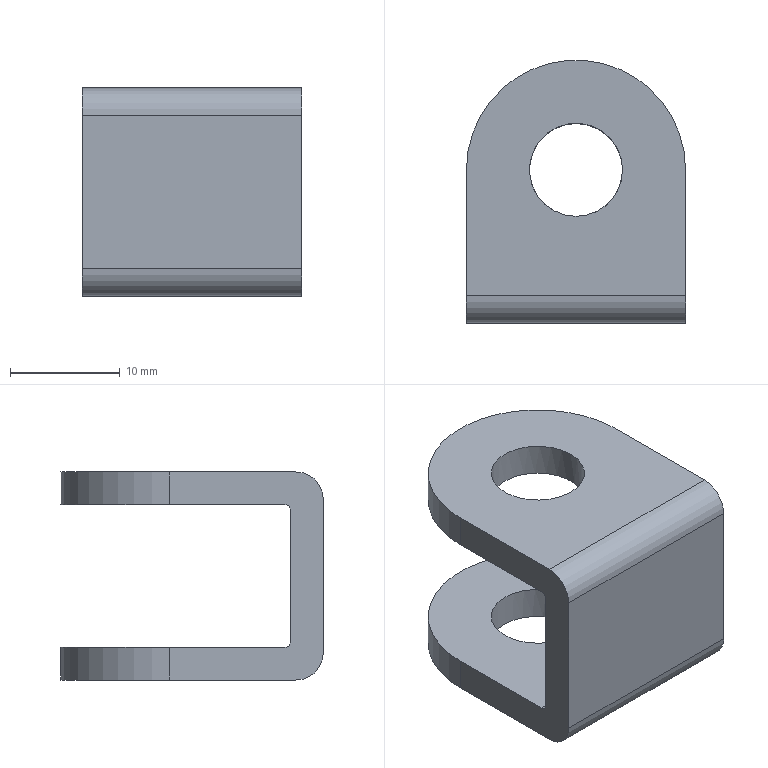Part | STEP file | PN_0023_default | 1 solid | 16 faces | box 20 x 24 x 19 mm | volume 3011 mm3 | cylinder 8 | plane 8 | commonest cylinder face diameters 1 x2 5 x2 8.5 x2 20 x2
STEP:
#1=CARTESIAN_POINT('',(0.,0.,0.));
#2=DIRECTION('',(0.,0.,1.));
#3=DIRECTION('',(1.,0.,0.));
#4=AXIS2_PLACEMENT_3D('',#1,#2,#3);
#5=CARTESIAN_POINT('',(10.,14.,9.5));
#6=VERTEX_POINT('',#5);
#7=CARTESIAN_POINT('',(10.,14.,6.5));
#8=VERTEX_POINT('',#7);
#9=CARTESIAN_POINT('',(10.,14.,9.5));
#10=DIRECTION('',(0.,0.,-1.));
#11=VECTOR('',#10,1.);
#12=LINE('',#9,#11);
#13=CARTESIAN_POINT('',(0.,14.,9.5));
#14=DIRECTION('',(0.,0.,-1.));
#15=DIRECTION('',(-1.,0.,0.));
#16=AXIS2_PLACEMENT_3D('',#13,#14,#15);
#17=CYLINDRICAL_SURFACE('',#16,10.);
#18=CARTESIAN_POINT('',(3.142,0.));
#19=DIRECTION('',(0.,1.));
#20=VECTOR('',#19,1.);
#21=LINE('',#18,#20);
#22=(GEOMETRIC_REPRESENTATION_CONTEXT(2)PARAMETRIC_REPRESENTATION_CONTEXT()REPRESENTATION_CONTEXT('',''));
#23=DEFINITIONAL_REPRESENTATION('',(#21),#22);
#24=PCURVE('',#17,#23);
#25=CARTESIAN_POINT('',(10.,0.,9.5));
#26=DIRECTION('',(-1.,0.,0.));
#27=DIRECTION('',(0.,-1.,0.));
#28=AXIS2_PLACEMENT_3D('',#25,#26,#27);
#29=PLANE('',#28);
#30=CARTESIAN_POINT('',(-14.,0.));
#31=DIRECTION('',(0.,-1.));
#32=VECTOR('',#31,1.);
#33=LINE('',#30,#32);
#34=(GEOMETRIC_REPRESENTATION_CONTEXT(2)PARAMETRIC_REPRESENTATION_CONTEXT()REPRESENTATION_CONTEXT('',''));
#35=DEFINITIONAL_REPRESENTATION('',(#33),#34);
#36=PCURVE('',#29,#35);
#37=SURFACE_CURVE('',#12,(#24,#36),.PCURVE_S1.);
#38=EDGE_CURVE('',#6,#8,#37,.T.);
#39=ORIENTED_EDGE('',*,*,#38,.T.);
#40=CARTESIAN_POINT('',(-10.,14.,6.5));
#41=VERTEX_POINT('',#40);
#42=CARTESIAN_POINT('',(0.,14.,6.5));
#43=DIRECTION('',(0.,0.,1.));
#44=DIRECTION('',(0.,-1.,0.));
#45=AXIS2_PLACEMENT_3D('',#42,#43,#44);
#46=CIRCLE('',#45,10.);
#47=CARTESIAN_POINT('',(4.712,3.));
#48=DIRECTION('',(-1.,0.));
#49=VECTOR('',#48,1.);
#50=LINE('',#47,#49);
#51=(GEOMETRIC_REPRESENTATION_CONTEXT(2)PARAMETRIC_REPRESENTATION_CONTEXT()REPRESENTATION_CONTEXT('',''));
#52=DEFINITIONAL_REPRESENTATION('',(#50),#51);
#53=PCURVE('',#17,#52);
#54=CARTESIAN_POINT('',(-10.,3.,6.5));
#55=DIRECTION('',(0.,0.,1.));
#56=DIRECTION('',(0.,-1.,0.));
#57=AXIS2_PLACEMENT_3D('',#54,#55,#56);
#58=PLANE('',#57);
#59=CARTESIAN_POINT('',(-11.,10.));
#60=DIRECTION('',(1.,0.));
#61=AXIS2_PLACEMENT_2D('',#59,#60);
#62=CIRCLE('',#61,10.);
#63=(GEOMETRIC_REPRESENTATION_CONTEXT(2)PARAMETRIC_REPRESENTATION_CONTEXT()REPRESENTATION_CONTEXT('',''));
#64=DEFINITIONAL_REPRESENTATION('',(#62),#63);
#65=PCURVE('',#58,#64);
#66=SURFACE_CURVE('',#46,(#53,#65),.PCURVE_S1.);
#67=EDGE_CURVE('',#8,#41,#66,.T.);
#68=ORIENTED_EDGE('',*,*,#67,.T.);
#69=CARTESIAN_POINT('',(-10.,14.,9.5));
#70=VERTEX_POINT('',#69);
#71=CARTESIAN_POINT('',(-10.,14.,9.5));
#72=DIRECTION('',(0.,0.,-1.));
#73=VECTOR('',#72,1.);
#74=LINE('',#71,#73);
#75=CARTESIAN_POINT('',(0.,0.));
#76=DIRECTION('',(0.,1.));
#77=VECTOR('',#76,1.);
#78=LINE('',#75,#77);
#79=(GEOMETRIC_REPRESENTATION_CONTEXT(2)PARAMETRIC_REPRESENTATION_CONTEXT()REPRESENTATION_CONTEXT('',''));
#80=DEFINITIONAL_REPRESENTATION('',(#78),#79);
#81=PCURVE('',#17,#80);
#82=CARTESIAN_POINT('',(-10.,0.,9.5));
#83=DIRECTION('',(1.,0.,0.));
#84=DIRECTION('',(0.,0.,-1.));
#85=AXIS2_PLACEMENT_3D('',#82,#83,#84);
#86=PLANE('',#85);
#87=CARTESIAN_POINT('',(0.,14.));
#88=DIRECTION('',(1.,0.));
#89=VECTOR('',#88,1.);
#90=LINE('',#87,#89);
#91=(GEOMETRIC_REPRESENTATION_CONTEXT(2)PARAMETRIC_REPRESENTATION_CONTEXT()REPRESENTATION_CONTEXT('',''));
#92=DEFINITIONAL_REPRESENTATION('',(#90),#91);
#93=PCURVE('',#86,#92);
#94=SURFACE_CURVE('',#74,(#81,#93),.PCURVE_S1.);
#95=EDGE_CURVE('',#70,#41,#94,.T.);
#96=ORIENTED_EDGE('',*,*,#95,.F.);
#97=CARTESIAN_POINT('',(0.,14.,9.5));
#98=DIRECTION('',(0.,0.,1.));
#99=DIRECTION('',(-1.,0.,0.));
#100=AXIS2_PLACEMENT_3D('',#97,#98,#99);
#101=CIRCLE('',#100,10.);
#102=CARTESIAN_POINT('',(6.283,0.));
#103=DIRECTION('',(-1.,0.));
#104=VECTOR('',#103,1.);
#105=LINE('',#102,#104);
#106=(GEOMETRIC_REPRESENTATION_CONTEXT(2)PARAMETRIC_REPRESENTATION_CONTEXT()REPRESENTATION_CONTEXT('',''));
#107=DEFINITIONAL_REPRESENTATION('',(#105),#106);
#108=PCURVE('',#17,#107);
#109=CARTESIAN_POINT('',(0.,14.,9.5));
#110=DIRECTION('',(0.,0.,-1.));
#111=DIRECTION('',(-1.,0.,0.));
#112=AXIS2_PLACEMENT_3D('',#109,#110,#111);
#113=PLANE('',#112);
#114=CARTESIAN_POINT('',(10.,0.));
#115=CARTESIAN_POINT('',(10.,-17.321));
#116=CARTESIAN_POINT('',(-5.,-8.66));
#117=CARTESIAN_POINT('',(-20.,0.));
#118=CARTESIAN_POINT('',(-5.,8.66));
#119=CARTESIAN_POINT('',(10.,17.321));
#120=CARTESIAN_POINT('',(10.,0.));
#121=(BOUNDED_CURVE()B_SPLINE_CURVE(2,(#114,#115,#116,#117,#118,#119,#120),.UNSPECIFIED.,.T.,.F.)B_SPLINE_CURVE_WITH_KNOTS((1,2,2,2,2,1),(-2.094,0.,2.094,4.189,6.283,8.378),.UNSPECIFIED.)CURVE()GEOMETRIC_REPRESENTATION_ITEM()RATIONAL_B_SPLINE_CURVE((1.,0.5,1.,0.5,1.,0.5,1.))REPRESENTATION_ITEM(''));
#122=(GEOMETRIC_REPRESENTATION_CONTEXT(2)PARAMETRIC_REPRESENTATION_CONTEXT()REPRESENTATION_CONTEXT('',''));
#123=DEFINITIONAL_REPRESENTATION('',(#121),#122);
#124=PCURVE('',#113,#123);
#125=SURFACE_CURVE('',#101,(#108,#124),.PCURVE_S1.);
#126=EDGE_CURVE('',#6,#70,#125,.T.);
#127=ORIENTED_EDGE('',*,*,#126,.F.);
#128=EDGE_LOOP('',(#39,#68,#96,#127));
#129=FACE_BOUND('',#128,.T.);
#130=ADVANCED_FACE('',(#129),#17,.T.);
#131=CARTESIAN_POINT('',(0.,9.75,6.5));
#132=VERTEX_POINT('',#131);
#133=CARTESIAN_POINT('',(0.,14.,6.5));
#134=DIRECTION('',(0.,0.,1.));
#135=DIRECTION('',(0.,-1.,0.));
#136=AXIS2_PLACEMENT_3D('',#133,#134,#135);
#137=CIRCLE('',#136,4.25);
#138=CARTESIAN_POINT('',(0.,14.,9.5));
#139=DIRECTION('',(0.,0.,-1.));
#140=DIRECTION('',(-1.,0.,0.));
#141=AXIS2_PLACEMENT_3D('',#138,#139,#140);
#142=CYLINDRICAL_SURFACE('',#141,4.25);
#143=CARTESIAN_POINT('',(10.996,3.));
#144=DIRECTION('',(-1.,0.));
#145=VECTOR('',#144,1.);
#146=LINE('',#143,#145);
#147=(GEOMETRIC_REPRESENTATION_CONTEXT(2)PARAMETRIC_REPRESENTATION_CONTEXT()REPRESENTATION_CONTEXT('',''));
#148=DEFINITIONAL_REPRESENTATION('',(#146),#147);
#149=PCURVE('',#142,#148);
#150=CARTESIAN_POINT('',(-11.,10.));
#151=DIRECTION('',(1.,0.));
#152=AXIS2_PLACEMENT_2D('',#150,#151);
#153=CIRCLE('',#152,4.25);
#154=(GEOMETRIC_REPRESENTATION_CONTEXT(2)PARAMETRIC_REPRESENTATION_CONTEXT()REPRESENTATION_CONTEXT('',''));
#155=DEFINITIONAL_REPRESENTATION('',(#153),#154);
#156=PCURVE('',#58,#155);
#157=SURFACE_CURVE('',#137,(#149,#156),.PCURVE_S1.);
#158=EDGE_CURVE('',#132,#132,#157,.T.);
#159=ORIENTED_EDGE('',*,*,#158,.T.);
#160=CARTESIAN_POINT('',(0.,9.75,9.5));
#161=VERTEX_POINT('',#160);
#162=CARTESIAN_POINT('',(0.,9.75,9.5));
#163=CARTESIAN_POINT('',(0.,9.75,6.5));
#164=B_SPLINE_CURVE_WITH_KNOTS('',1,(#162,#163),.UNSPECIFIED.,.F.,.F.,(2,2),(0.,3.),.PIECEWISE_BEZIER_KNOTS.);
#165=CARTESIAN_POINT('',(4.712,0.));
#166=DIRECTION('',(0.,1.));
#167=VECTOR('',#166,1.);
#168=LINE('',#165,#167);
#169=(GEOMETRIC_REPRESENTATION_CONTEXT(2)PARAMETRIC_REPRESENTATION_CONTEXT()REPRESENTATION_CONTEXT('',''));
#170=DEFINITIONAL_REPRESENTATION('',(#168),#169);
#171=PCURVE('',#142,#170);
#172=CARTESIAN_POINT('',(10.996,0.));
#173=DIRECTION('',(0.,1.));
#174=VECTOR('',#173,1.);
#175=LINE('',#172,#174);
#176=(GEOMETRIC_REPRESENTATION_CONTEXT(2)PARAMETRIC_REPRESENTATION_CONTEXT()REPRESENTATION_CONTEXT('',''));
#177=DEFINITIONAL_REPRESENTATION('',(#175),#176);
#178=PCURVE('',#142,#177);
#179=SEAM_CURVE('',#164,(#171,#178),.PCURVE_S1.);
#180=EDGE_CURVE('',#161,#132,#179,.T.);
#181=ORIENTED_EDGE('',*,*,#180,.F.);
#182=CARTESIAN_POINT('',(4.25,14.,9.5));
#183=VERTEX_POINT('',#182);
#184=CARTESIAN_POINT('',(0.,14.,9.5));
#185=DIRECTION('',(0.,0.,1.));
#186=DIRECTION('',(1.,0.,0.));
#187=AXIS2_PLACEMENT_3D('',#184,#185,#186);
#188=CIRCLE('',#187,4.25);
#189=CARTESIAN_POINT('',(9.425,0.));
#190=DIRECTION('',(-1.,0.));
#191=VECTOR('',#190,1.);
#192=LINE('',#189,#191);
#193=(GEOMETRIC_REPRESENTATION_CONTEXT(2)PARAMETRIC_REPRESENTATION_CONTEXT()REPRESENTATION_CONTEXT('',''));
#194=DEFINITIONAL_REPRESENTATION('',(#192),#193);
#195=PCURVE('',#142,#194);
#196=CARTESIAN_POINT('',(-4.25,0.));
#197=CARTESIAN_POINT('',(-4.25,7.361));
#198=CARTESIAN_POINT('',(2.125,3.681));
#199=CARTESIAN_POINT('',(8.5,0.));
#200=CARTESIAN_POINT('',(2.125,-3.681));
#201=CARTESIAN_POINT('',(-4.25,-7.361));
#202=CARTESIAN_POINT('',(-4.25,0.));
#203=(BOUNDED_CURVE()B_SPLINE_CURVE(2,(#196,#197,#198,#199,#200,#201,#202),.UNSPECIFIED.,.T.,.F.)B_SPLINE_CURVE_WITH_KNOTS((1,2,2,2,2,1),(-2.094,0.,2.094,4.189,6.283,8.378),.UNSPECIFIED.)CURVE()GEOMETRIC_REPRESENTATION_ITEM()RATIONAL_B_SPLINE_CURVE((1.,0.5,1.,0.5,1.,0.5,1.))REPRESENTATION_ITEM(''));
#204=(GEOMETRIC_REPRESENTATION_CONTEXT(2)PARAMETRIC_REPRESENTATION_CONTEXT()REPRESENTATION_CONTEXT('',''));
#205=DEFINITIONAL_REPRESENTATION('',(#203),#204);
#206=PCURVE('',#113,#205);
#207=SURFACE_CURVE('',#188,(#195,#206),.PCURVE_S1.);
#208=EDGE_CURVE('',#183,#161,#207,.T.);
#209=ORIENTED_EDGE('',*,*,#208,.F.);
#210=CARTESIAN_POINT('',(0.,14.,9.5));
#211=DIRECTION('',(0.,0.,1.));
#212=DIRECTION('',(1.,0.,0.));
#213=AXIS2_PLACEMENT_3D('',#210,#211,#212);
#214=CIRCLE('',#213,4.25);
#215=CARTESIAN_POINT('',(15.708,0.));
#216=DIRECTION('',(-1.,0.));
#217=VECTOR('',#216,1.);
#218=LINE('',#215,#217);
#219=(GEOMETRIC_REPRESENTATION_CONTEXT(2)PARAMETRIC_REPRESENTATION_CONTEXT()REPRESENTATION_CONTEXT('',''));
#220=DEFINITIONAL_REPRESENTATION('',(#218),#219);
#221=PCURVE('',#142,#220);
#222=CARTESIAN_POINT('',(-4.25,0.));
#223=CARTESIAN_POINT('',(-4.25,7.361));
#224=CARTESIAN_POINT('',(2.125,3.681));
#225=CARTESIAN_POINT('',(8.5,0.));
#226=CARTESIAN_POINT('',(2.125,-3.681));
#227=CARTESIAN_POINT('',(-4.25,-7.361));
#228=CARTESIAN_POINT('',(-4.25,0.));
#229=(BOUNDED_CURVE()B_SPLINE_CURVE(2,(#222,#223,#224,#225,#226,#227,#228),.UNSPECIFIED.,.T.,.F.)B_SPLINE_CURVE_WITH_KNOTS((1,2,2,2,2,1),(-2.094,0.,2.094,4.189,6.283,8.378),.UNSPECIFIED.)CURVE()GEOMETRIC_REPRESENTATION_ITEM()RATIONAL_B_SPLINE_CURVE((1.,0.5,1.,0.5,1.,0.5,1.))REPRESENTATION_ITEM(''));
#230=(GEOMETRIC_REPRESENTATION_CONTEXT(2)PARAMETRIC_REPRESENTATION_CONTEXT()REPRESENTATION_CONTEXT('',''));
#231=DEFINITIONAL_REPRESENTATION('',(#229),#230);
#232=PCURVE('',#113,#231);
#233=SURFACE_CURVE('',#214,(#221,#232),.PCURVE_S1.);
#234=EDGE_CURVE('',#161,#183,#233,.T.);
#235=ORIENTED_EDGE('',*,*,#234,.F.);
#236=ORIENTED_EDGE('',*,*,#180,.T.);
#237=EDGE_LOOP('',(#159,#181,#209,#235,#236));
#238=FACE_BOUND('',#237,.F.);
#239=ADVANCED_FACE('',(#238),#142,.F.);
#240=CARTESIAN_POINT('',(-10.,2.5,9.5));
#241=VERTEX_POINT('',#240);
#242=CARTESIAN_POINT('',(-10.,0.,9.5));
#243=DIRECTION('',(0.,-1.,0.));
#244=VECTOR('',#243,1.);
#245=LINE('',#242,#244);
#246=CARTESIAN_POINT('',(10.,-14.));
#247=DIRECTION('',(0.,-1.));
#248=VECTOR('',#247,1.);
#249=LINE('',#246,#248);
#250=(GEOMETRIC_REPRESENTATION_CONTEXT(2)PARAMETRIC_REPRESENTATION_CONTEXT()REPRESENTATION_CONTEXT('',''));
#251=DEFINITIONAL_REPRESENTATION('',(#249),#250);
#252=PCURVE('',#113,#251);
#253=CARTESIAN_POINT('',(0.,0.));
#254=DIRECTION('',(0.,-1.));
#255=VECTOR('',#254,1.);
#256=LINE('',#253,#255);
#257=(GEOMETRIC_REPRESENTATION_CONTEXT(2)PARAMETRIC_REPRESENTATION_CONTEXT()REPRESENTATION_CONTEXT('',''));
#258=DEFINITIONAL_REPRESENTATION('',(#256),#257);
#259=PCURVE('',#86,#258);
#260=SURFACE_CURVE('',#245,(#252,#259),.PCURVE_S1.);
#261=EDGE_CURVE('',#70,#241,#260,.T.);
#262=ORIENTED_EDGE('',*,*,#261,.T.);
#263=CARTESIAN_POINT('',(10.,2.5,9.5));
#264=VERTEX_POINT('',#263);
#265=CARTESIAN_POINT('',(0.,2.5,9.5));
#266=DIRECTION('',(1.,0.,0.));
#267=VECTOR('',#266,1.);
#268=LINE('',#265,#267);
#269=CARTESIAN_POINT('',(0.,-11.5));
#270=DIRECTION('',(-1.,0.));
#271=VECTOR('',#270,1.);
#272=LINE('',#269,#271);
#273=(GEOMETRIC_REPRESENTATION_CONTEXT(2)PARAMETRIC_REPRESENTATION_CONTEXT()REPRESENTATION_CONTEXT('',''));
#274=DEFINITIONAL_REPRESENTATION('',(#272),#273);
#275=PCURVE('',#113,#274);
#276=CARTESIAN_POINT('',(0.,2.5,7.));
#277=DIRECTION('',(1.,0.,0.));
#278=DIRECTION('',(0.,1.,0.));
#279=AXIS2_PLACEMENT_3D('',#276,#277,#278);
#280=CYLINDRICAL_SURFACE('',#279,2.5);
#281=CARTESIAN_POINT('',(1.571,0.));
#282=DIRECTION('',(0.,1.));
#283=VECTOR('',#282,1.);
#284=LINE('',#281,#283);
#285=(GEOMETRIC_REPRESENTATION_CONTEXT(2)PARAMETRIC_REPRESENTATION_CONTEXT()REPRESENTATION_CONTEXT('',''));
#286=DEFINITIONAL_REPRESENTATION('',(#284),#285);
#287=PCURVE('',#280,#286);
#288=SURFACE_CURVE('',#268,(#275,#287),.PCURVE_S1.);
#289=EDGE_CURVE('',#241,#264,#288,.T.);
#290=ORIENTED_EDGE('',*,*,#289,.T.);
#291=CARTESIAN_POINT('',(10.,0.,9.5));
#292=DIRECTION('',(0.,1.,0.));
#293=VECTOR('',#292,1.);
#294=LINE('',#291,#293);
#295=CARTESIAN_POINT('',(-10.,-14.));
#296=DIRECTION('',(0.,1.));
#297=VECTOR('',#296,1.);
#298=LINE('',#295,#297);
#299=(GEOMETRIC_REPRESENTATION_CONTEXT(2)PARAMETRIC_REPRESENTATION_CONTEXT()REPRESENTATION_CONTEXT('',''));
#300=DEFINITIONAL_REPRESENTATION('',(#298),#299);
#301=PCURVE('',#113,#300);
#302=CARTESIAN_POINT('',(0.,0.));
#303=DIRECTION('',(-1.,0.));
#304=VECTOR('',#303,1.);
#305=LINE('',#302,#304);
#306=(GEOMETRIC_REPRESENTATION_CONTEXT(2)PARAMETRIC_REPRESENTATION_CONTEXT()REPRESENTATION_CONTEXT('',''));
#307=DEFINITIONAL_REPRESENTATION('',(#305),#306);
#308=PCURVE('',#29,#307);
#309=SURFACE_CURVE('',#294,(#301,#308),.PCURVE_S1.);
#310=EDGE_CURVE('',#264,#6,#309,.T.);
#311=ORIENTED_EDGE('',*,*,#310,.T.);
#312=ORIENTED_EDGE('',*,*,#126,.T.);
#313=EDGE_LOOP('',(#262,#290,#311,#312));
#314=FACE_BOUND('',#313,.T.);
#315=ORIENTED_EDGE('',*,*,#208,.F.);
#316=ORIENTED_EDGE('',*,*,#234,.F.);
#317=EDGE_LOOP('',(#315,#316));
#318=FACE_BOUND('',#317,.T.);
#319=ADVANCED_FACE('',(#314,#318),#113,.F.);
#320=CARTESIAN_POINT('',(10.,2.5,-9.5));
#321=VERTEX_POINT('',#320);
#322=CARTESIAN_POINT('',(10.,14.,-9.5));
#323=VERTEX_POINT('',#322);
#324=CARTESIAN_POINT('',(10.,0.,-9.5));
#325=DIRECTION('',(0.,1.,0.));
#326=VECTOR('',#325,1.);
#327=LINE('',#324,#326);
#328=CARTESIAN_POINT('',(0.,14.,-9.5));
#329=DIRECTION('',(0.,0.,-1.));
#330=DIRECTION('',(-1.,0.,0.));
#331=AXIS2_PLACEMENT_3D('',#328,#329,#330);
#332=PLANE('',#331);
#333=CARTESIAN_POINT('',(-10.,-14.));
#334=DIRECTION('',(0.,1.));
#335=VECTOR('',#334,1.);
#336=LINE('',#333,#335);
#337=(GEOMETRIC_REPRESENTATION_CONTEXT(2)PARAMETRIC_REPRESENTATION_CONTEXT()REPRESENTATION_CONTEXT('',''));
#338=DEFINITIONAL_REPRESENTATION('',(#336),#337);
#339=PCURVE('',#332,#338);
#340=CARTESIAN_POINT('',(0.,-19.));
#341=DIRECTION('',(-1.,0.));
#342=VECTOR('',#341,1.);
#343=LINE('',#340,#342);
#344=(GEOMETRIC_REPRESENTATION_CONTEXT(2)PARAMETRIC_REPRESENTATION_CONTEXT()REPRESENTATION_CONTEXT('',''));
#345=DEFINITIONAL_REPRESENTATION('',(#343),#344);
#346=PCURVE('',#29,#345);
#347=SURFACE_CURVE('',#327,(#339,#346),.PCURVE_S1.);
#348=EDGE_CURVE('',#321,#323,#347,.T.);
#349=ORIENTED_EDGE('',*,*,#348,.F.);
#350=CARTESIAN_POINT('',(-10.,2.5,-9.5));
#351=VERTEX_POINT('',#350);
#352=CARTESIAN_POINT('',(-10.,2.5,-9.5));
#353=DIRECTION('',(-1.,0.,0.));
#354=VECTOR('',#353,1.);
#355=LINE('',#352,#354);
#356=CARTESIAN_POINT('',(10.,-11.5));
#357=DIRECTION('',(1.,0.));
#358=VECTOR('',#357,1.);
#359=LINE('',#356,#358);
#360=(GEOMETRIC_REPRESENTATION_CONTEXT(2)PARAMETRIC_REPRESENTATION_CONTEXT()REPRESENTATION_CONTEXT('',''));
#361=DEFINITIONAL_REPRESENTATION('',(#359),#360);
#362=PCURVE('',#332,#361);
#363=CARTESIAN_POINT('',(-10.,2.5,-7.));
#364=DIRECTION('',(-1.,0.,0.));
#365=DIRECTION('',(0.,-1.,0.));
#366=AXIS2_PLACEMENT_3D('',#363,#364,#365);
#367=CYLINDRICAL_SURFACE('',#366,2.5);
#368=CARTESIAN_POINT('',(4.712,0.));
#369=DIRECTION('',(0.,1.));
#370=VECTOR('',#369,1.);
#371=LINE('',#368,#370);
#372=(GEOMETRIC_REPRESENTATION_CONTEXT(2)PARAMETRIC_REPRESENTATION_CONTEXT()REPRESENTATION_CONTEXT('',''));
#373=DEFINITIONAL_REPRESENTATION('',(#371),#372);
#374=PCURVE('',#367,#373);
#375=SURFACE_CURVE('',#355,(#362,#374),.PCURVE_S1.);
#376=EDGE_CURVE('',#321,#351,#375,.T.);
#377=ORIENTED_EDGE('',*,*,#376,.T.);
#378=CARTESIAN_POINT('',(-10.,14.,-9.5));
#379=VERTEX_POINT('',#378);
#380=CARTESIAN_POINT('',(-10.,0.,-9.5));
#381=DIRECTION('',(0.,-1.,0.));
#382=VECTOR('',#381,1.);
#383=LINE('',#380,#382);
#384=CARTESIAN_POINT('',(10.,-14.));
#385=DIRECTION('',(0.,-1.));
#386=VECTOR('',#385,1.);
#387=LINE('',#384,#386);
#388=(GEOMETRIC_REPRESENTATION_CONTEXT(2)PARAMETRIC_REPRESENTATION_CONTEXT()REPRESENTATION_CONTEXT('',''));
#389=DEFINITIONAL_REPRESENTATION('',(#387),#388);
#390=PCURVE('',#332,#389);
#391=CARTESIAN_POINT('',(19.,0.));
#392=DIRECTION('',(0.,-1.));
#393=VECTOR('',#392,1.);
#394=LINE('',#391,#393);
#395=(GEOMETRIC_REPRESENTATION_CONTEXT(2)PARAMETRIC_REPRESENTATION_CONTEXT()REPRESENTATION_CONTEXT('',''));
#396=DEFINITIONAL_REPRESENTATION('',(#394),#395);
#397=PCURVE('',#86,#396);
#398=SURFACE_CURVE('',#383,(#390,#397),.PCURVE_S1.);
#399=EDGE_CURVE('',#379,#351,#398,.T.);
#400=ORIENTED_EDGE('',*,*,#399,.F.);
#401=CARTESIAN_POINT('',(0.,14.,-9.5));
#402=DIRECTION('',(0.,0.,1.));
#403=DIRECTION('',(-1.,0.,0.));
#404=AXIS2_PLACEMENT_3D('',#401,#402,#403);
#405=CIRCLE('',#404,10.);
#406=CARTESIAN_POINT('',(10.,0.));
#407=CARTESIAN_POINT('',(10.,-17.321));
#408=CARTESIAN_POINT('',(-5.,-8.66));
#409=CARTESIAN_POINT('',(-20.,0.));
#410=CARTESIAN_POINT('',(-5.,8.66));
#411=CARTESIAN_POINT('',(10.,17.321));
#412=CARTESIAN_POINT('',(10.,0.));
#413=(BOUNDED_CURVE()B_SPLINE_CURVE(2,(#406,#407,#408,#409,#410,#411,#412),.UNSPECIFIED.,.T.,.F.)B_SPLINE_CURVE_WITH_KNOTS((1,2,2,2,2,1),(-2.094,0.,2.094,4.189,6.283,8.378),.UNSPECIFIED.)CURVE()GEOMETRIC_REPRESENTATION_ITEM()RATIONAL_B_SPLINE_CURVE((1.,0.5,1.,0.5,1.,0.5,1.))REPRESENTATION_ITEM(''));
#414=(GEOMETRIC_REPRESENTATION_CONTEXT(2)PARAMETRIC_REPRESENTATION_CONTEXT()REPRESENTATION_CONTEXT('',''));
#415=DEFINITIONAL_REPRESENTATION('',(#413),#414);
#416=PCURVE('',#332,#415);
#417=CARTESIAN_POINT('',(0.,14.,9.5));
#418=DIRECTION('',(0.,0.,-1.));
#419=DIRECTION('',(-1.,0.,0.));
#420=AXIS2_PLACEMENT_3D('',#417,#418,#419);
#421=CYLINDRICAL_SURFACE('',#420,10.);
#422=CARTESIAN_POINT('',(6.283,19.));
#423=DIRECTION('',(-1.,0.));
#424=VECTOR('',#423,1.);
#425=LINE('',#422,#424);
#426=(GEOMETRIC_REPRESENTATION_CONTEXT(2)PARAMETRIC_REPRESENTATION_CONTEXT()REPRESENTATION_CONTEXT('',''));
#427=DEFINITIONAL_REPRESENTATION('',(#425),#426);
#428=PCURVE('',#421,#427);
#429=SURFACE_CURVE('',#405,(#416,#428),.PCURVE_S1.);
#430=EDGE_CURVE('',#323,#379,#429,.T.);
#431=ORIENTED_EDGE('',*,*,#430,.F.);
#432=EDGE_LOOP('',(#349,#377,#400,#431));
#433=FACE_BOUND('',#432,.T.);
#434=CARTESIAN_POINT('',(4.25,14.,-9.5));
#435=VERTEX_POINT('',#434);
#436=CARTESIAN_POINT('',(0.,18.25,-9.5));
#437=VERTEX_POINT('',#436);
#438=CARTESIAN_POINT('',(0.,14.,-9.5));
#439=DIRECTION('',(0.,0.,1.));
#440=DIRECTION('',(1.,0.,0.));
#441=AXIS2_PLACEMENT_3D('',#438,#439,#440);
#442=CIRCLE('',#441,4.25);
#443=CARTESIAN_POINT('',(-4.25,0.));
#444=CARTESIAN_POINT('',(-4.25,7.361));
#445=CARTESIAN_POINT('',(2.125,3.681));
#446=CARTESIAN_POINT('',(8.5,0.));
#447=CARTESIAN_POINT('',(2.125,-3.681));
#448=CARTESIAN_POINT('',(-4.25,-7.361));
#449=CARTESIAN_POINT('',(-4.25,0.));
#450=(BOUNDED_CURVE()B_SPLINE_CURVE(2,(#443,#444,#445,#446,#447,#448,#449),.UNSPECIFIED.,.T.,.F.)B_SPLINE_CURVE_WITH_KNOTS((1,2,2,2,2,1),(-2.094,0.,2.094,4.189,6.283,8.378),.UNSPECIFIED.)CURVE()GEOMETRIC_REPRESENTATION_ITEM()RATIONAL_B_SPLINE_CURVE((1.,0.5,1.,0.5,1.,0.5,1.))REPRESENTATION_ITEM(''));
#451=(GEOMETRIC_REPRESENTATION_CONTEXT(2)PARAMETRIC_REPRESENTATION_CONTEXT()REPRESENTATION_CONTEXT('',''));
#452=DEFINITIONAL_REPRESENTATION('',(#450),#451);
#453=PCURVE('',#332,#452);
#454=CARTESIAN_POINT('',(0.,14.,9.5));
#455=DIRECTION('',(0.,0.,-1.));
#456=DIRECTION('',(-1.,0.,0.));
#457=AXIS2_PLACEMENT_3D('',#454,#455,#456);
#458=CYLINDRICAL_SURFACE('',#457,4.25);
#459=CARTESIAN_POINT('',(3.142,19.));
#460=DIRECTION('',(-1.,0.));
#461=VECTOR('',#460,1.);
#462=LINE('',#459,#461);
#463=(GEOMETRIC_REPRESENTATION_CONTEXT(2)PARAMETRIC_REPRESENTATION_CONTEXT()REPRESENTATION_CONTEXT('',''));
#464=DEFINITIONAL_REPRESENTATION('',(#462),#463);
#465=PCURVE('',#458,#464);
#466=SURFACE_CURVE('',#442,(#453,#465),.PCURVE_S1.);
#467=EDGE_CURVE('',#435,#437,#466,.T.);
#468=ORIENTED_EDGE('',*,*,#467,.T.);
#469=CARTESIAN_POINT('',(0.,14.,-9.5));
#470=DIRECTION('',(0.,0.,1.));
#471=DIRECTION('',(1.,0.,0.));
#472=AXIS2_PLACEMENT_3D('',#469,#470,#471);
#473=CIRCLE('',#472,4.25);
#474=CARTESIAN_POINT('',(-4.25,0.));
#475=CARTESIAN_POINT('',(-4.25,7.361));
#476=CARTESIAN_POINT('',(2.125,3.681));
#477=CARTESIAN_POINT('',(8.5,0.));
#478=CARTESIAN_POINT('',(2.125,-3.681));
#479=CARTESIAN_POINT('',(-4.25,-7.361));
#480=CARTESIAN_POINT('',(-4.25,0.));
#481=(BOUNDED_CURVE()B_SPLINE_CURVE(2,(#474,#475,#476,#477,#478,#479,#480),.UNSPECIFIED.,.T.,.F.)B_SPLINE_CURVE_WITH_KNOTS((1,2,2,2,2,1),(-2.094,0.,2.094,4.189,6.283,8.378),.UNSPECIFIED.)CURVE()GEOMETRIC_REPRESENTATION_ITEM()RATIONAL_B_SPLINE_CURVE((1.,0.5,1.,0.5,1.,0.5,1.))REPRESENTATION_ITEM(''));
#482=(GEOMETRIC_REPRESENTATION_CONTEXT(2)PARAMETRIC_REPRESENTATION_CONTEXT()REPRESENTATION_CONTEXT('',''));
#483=DEFINITIONAL_REPRESENTATION('',(#481),#482);
#484=PCURVE('',#332,#483);
#485=CARTESIAN_POINT('',(9.425,19.));
#486=DIRECTION('',(-1.,0.));
#487=VECTOR('',#486,1.);
#488=LINE('',#485,#487);
#489=(GEOMETRIC_REPRESENTATION_CONTEXT(2)PARAMETRIC_REPRESENTATION_CONTEXT()REPRESENTATION_CONTEXT('',''));
#490=DEFINITIONAL_REPRESENTATION('',(#488),#489);
#491=PCURVE('',#458,#490);
#492=SURFACE_CURVE('',#473,(#484,#491),.PCURVE_S1.);
#493=EDGE_CURVE('',#437,#435,#492,.T.);
#494=ORIENTED_EDGE('',*,*,#493,.T.);
#495=EDGE_LOOP('',(#468,#494));
#496=FACE_BOUND('',#495,.T.);
#497=ADVANCED_FACE('',(#433,#496),#332,.T.);
#498=CARTESIAN_POINT('',(-10.,0.,7.));
#499=VERTEX_POINT('',#498);
#500=CARTESIAN_POINT('',(-10.,0.,-7.));
#501=VERTEX_POINT('',#500);
#502=CARTESIAN_POINT('',(-10.,0.,9.5));
#503=DIRECTION('',(0.,0.,-1.));
#504=VECTOR('',#503,1.);
#505=LINE('',#502,#504);
#506=CARTESIAN_POINT('',(-10.,0.,9.5));
#507=DIRECTION('',(0.,1.,0.));
#508=DIRECTION('',(-1.,0.,0.));
#509=AXIS2_PLACEMENT_3D('',#506,#507,#508);
#510=PLANE('',#509);
#511=CARTESIAN_POINT('',(0.,0.));
#512=DIRECTION('',(0.,-1.));
#513=VECTOR('',#512,1.);
#514=LINE('',#511,#513);
#515=(GEOMETRIC_REPRESENTATION_CONTEXT(2)PARAMETRIC_REPRESENTATION_CONTEXT()REPRESENTATION_CONTEXT('',''));
#516=DEFINITIONAL_REPRESENTATION('',(#514),#515);
#517=PCURVE('',#510,#516);
#518=CARTESIAN_POINT('',(0.,0.));
#519=DIRECTION('',(1.,0.));
#520=VECTOR('',#519,1.);
#521=LINE('',#518,#520);
#522=(GEOMETRIC_REPRESENTATION_CONTEXT(2)PARAMETRIC_REPRESENTATION_CONTEXT()REPRESENTATION_CONTEXT('',''));
#523=DEFINITIONAL_REPRESENTATION('',(#521),#522);
#524=PCURVE('',#86,#523);
#525=SURFACE_CURVE('',#505,(#517,#524),.PCURVE_S1.);
#526=EDGE_CURVE('',#499,#501,#525,.T.);
#527=ORIENTED_EDGE('',*,*,#526,.T.);
#528=CARTESIAN_POINT('',(10.,0.,-7.));
#529=VERTEX_POINT('',#528);
#530=CARTESIAN_POINT('',(10.,0.,-7.));
#531=DIRECTION('',(1.,0.,0.));
#532=VECTOR('',#531,1.);
#533=LINE('',#530,#532);
#534=CARTESIAN_POINT('',(-20.,-16.5));
#535=DIRECTION('',(-1.,0.));
#536=VECTOR('',#535,1.);
#537=LINE('',#534,#536);
#538=(GEOMETRIC_REPRESENTATION_CONTEXT(2)PARAMETRIC_REPRESENTATION_CONTEXT()REPRESENTATION_CONTEXT('',''));
#539=DEFINITIONAL_REPRESENTATION('',(#537),#538);
#540=PCURVE('',#510,#539);
#541=CARTESIAN_POINT('',(6.283,-20.));
#542=DIRECTION('',(0.,-1.));
#543=VECTOR('',#542,1.);
#544=LINE('',#541,#543);
#545=(GEOMETRIC_REPRESENTATION_CONTEXT(2)PARAMETRIC_REPRESENTATION_CONTEXT()REPRESENTATION_CONTEXT('',''));
#546=DEFINITIONAL_REPRESENTATION('',(#544),#545);
#547=PCURVE('',#367,#546);
#548=SURFACE_CURVE('',#533,(#540,#547),.PCURVE_S1.);
#549=EDGE_CURVE('',#501,#529,#548,.T.);
#550=ORIENTED_EDGE('',*,*,#549,.T.);
#551=CARTESIAN_POINT('',(10.,0.,7.));
#552=VERTEX_POINT('',#551);
#553=CARTESIAN_POINT('',(10.,0.,9.5));
#554=DIRECTION('',(0.,0.,-1.));
#555=VECTOR('',#554,1.);
#556=LINE('',#553,#555);
#557=CARTESIAN_POINT('',(-20.,0.));
#558=DIRECTION('',(0.,-1.));
#559=VECTOR('',#558,1.);
#560=LINE('',#557,#559);
#561=(GEOMETRIC_REPRESENTATION_CONTEXT(2)PARAMETRIC_REPRESENTATION_CONTEXT()REPRESENTATION_CONTEXT('',''));
#562=DEFINITIONAL_REPRESENTATION('',(#560),#561);
#563=PCURVE('',#510,#562);
#564=CARTESIAN_POINT('',(0.,0.));
#565=DIRECTION('',(0.,-1.));
#566=VECTOR('',#565,1.);
#567=LINE('',#564,#566);
#568=(GEOMETRIC_REPRESENTATION_CONTEXT(2)PARAMETRIC_REPRESENTATION_CONTEXT()REPRESENTATION_CONTEXT('',''));
#569=DEFINITIONAL_REPRESENTATION('',(#567),#568);
#570=PCURVE('',#29,#569);
#571=SURFACE_CURVE('',#556,(#563,#570),.PCURVE_S1.);
#572=EDGE_CURVE('',#552,#529,#571,.T.);
#573=ORIENTED_EDGE('',*,*,#572,.F.);
#574=CARTESIAN_POINT('',(-10.,0.,7.));
#575=DIRECTION('',(-1.,0.,0.));
#576=VECTOR('',#575,1.);
#577=LINE('',#574,#576);
#578=CARTESIAN_POINT('',(0.,-2.5));
#579=DIRECTION('',(1.,0.));
#580=VECTOR('',#579,1.);
#581=LINE('',#578,#580);
#582=(GEOMETRIC_REPRESENTATION_CONTEXT(2)PARAMETRIC_REPRESENTATION_CONTEXT()REPRESENTATION_CONTEXT('',''));
#583=DEFINITIONAL_REPRESENTATION('',(#581),#582);
#584=PCURVE('',#510,#583);
#585=CARTESIAN_POINT('',(3.142,-10.));
#586=DIRECTION('',(0.,-1.));
#587=VECTOR('',#586,1.);
#588=LINE('',#585,#587);
#589=(GEOMETRIC_REPRESENTATION_CONTEXT(2)PARAMETRIC_REPRESENTATION_CONTEXT()REPRESENTATION_CONTEXT('',''));
#590=DEFINITIONAL_REPRESENTATION('',(#588),#589);
#591=PCURVE('',#280,#590);
#592=SURFACE_CURVE('',#577,(#584,#591),.PCURVE_S1.);
#593=EDGE_CURVE('',#552,#499,#592,.T.);
#594=ORIENTED_EDGE('',*,*,#593,.T.);
#595=EDGE_LOOP('',(#527,#550,#573,#594));
#596=FACE_BOUND('',#595,.T.);
#597=ADVANCED_FACE('',(#596),#510,.F.);
#598=ORIENTED_EDGE('',*,*,#572,.T.);
#599=CARTESIAN_POINT('',(10.,2.5,-7.));
#600=DIRECTION('',(1.,0.,0.));
#601=DIRECTION('',(0.,-1.,0.));
#602=AXIS2_PLACEMENT_3D('',#599,#600,#601);
#603=CIRCLE('',#602,2.5);
#604=CARTESIAN_POINT('',(0.,-16.5));
#605=CARTESIAN_POINT('',(0.,-20.83));
#606=CARTESIAN_POINT('',(-3.75,-18.665));
#607=CARTESIAN_POINT('',(-7.5,-16.5));
#608=CARTESIAN_POINT('',(-3.75,-14.335));
#609=CARTESIAN_POINT('',(0.,-12.17));
#610=CARTESIAN_POINT('',(0.,-16.5));
#611=(BOUNDED_CURVE()B_SPLINE_CURVE(2,(#604,#605,#606,#607,#608,#609,#610),.UNSPECIFIED.,.T.,.F.)B_SPLINE_CURVE_WITH_KNOTS((1,2,2,2,2,1),(-2.094,0.,2.094,4.189,6.283,8.378),.UNSPECIFIED.)CURVE()GEOMETRIC_REPRESENTATION_ITEM()RATIONAL_B_SPLINE_CURVE((1.,0.5,1.,0.5,1.,0.5,1.))REPRESENTATION_ITEM(''));
#612=(GEOMETRIC_REPRESENTATION_CONTEXT(2)PARAMETRIC_REPRESENTATION_CONTEXT()REPRESENTATION_CONTEXT('',''));
#613=DEFINITIONAL_REPRESENTATION('',(#611),#612);
#614=PCURVE('',#29,#613);
#615=CARTESIAN_POINT('',(6.283,-20.));
#616=DIRECTION('',(-1.,0.));
#617=VECTOR('',#616,1.);
#618=LINE('',#615,#617);
#619=(GEOMETRIC_REPRESENTATION_CONTEXT(2)PARAMETRIC_REPRESENTATION_CONTEXT()REPRESENTATION_CONTEXT('',''));
#620=DEFINITIONAL_REPRESENTATION('',(#618),#619);
#621=PCURVE('',#367,#620);
#622=SURFACE_CURVE('',#603,(#614,#621),.PCURVE_S1.);
#623=EDGE_CURVE('',#529,#321,#622,.T.);
#624=ORIENTED_EDGE('',*,*,#623,.T.);
#625=ORIENTED_EDGE('',*,*,#348,.T.);
#626=CARTESIAN_POINT('',(10.,14.,-6.5));
#627=VERTEX_POINT('',#626);
#628=CARTESIAN_POINT('',(10.,14.,9.5));
#629=DIRECTION('',(0.,0.,-1.));
#630=VECTOR('',#629,1.);
#631=LINE('',#628,#630);
#632=CARTESIAN_POINT('',(-14.,0.));
#633=DIRECTION('',(0.,-1.));
#634=VECTOR('',#633,1.);
#635=LINE('',#632,#634);
#636=(GEOMETRIC_REPRESENTATION_CONTEXT(2)PARAMETRIC_REPRESENTATION_CONTEXT()REPRESENTATION_CONTEXT('',''));
#637=DEFINITIONAL_REPRESENTATION('',(#635),#636);
#638=PCURVE('',#29,#637);
#639=CARTESIAN_POINT('',(3.142,0.));
#640=DIRECTION('',(0.,1.));
#641=VECTOR('',#640,1.);
#642=LINE('',#639,#641);
#643=(GEOMETRIC_REPRESENTATION_CONTEXT(2)PARAMETRIC_REPRESENTATION_CONTEXT()REPRESENTATION_CONTEXT('',''));
#644=DEFINITIONAL_REPRESENTATION('',(#642),#643);
#645=PCURVE('',#421,#644);
#646=SURFACE_CURVE('',#631,(#638,#645),.PCURVE_S1.);
#647=EDGE_CURVE('',#627,#323,#646,.T.);
#648=ORIENTED_EDGE('',*,*,#647,.F.);
#649=CARTESIAN_POINT('',(10.,3.5,-6.5));
#650=VERTEX_POINT('',#649);
#651=CARTESIAN_POINT('',(10.,3.,-6.5));
#652=DIRECTION('',(0.,1.,0.));
#653=VECTOR('',#652,1.);
#654=LINE('',#651,#653);
#655=CARTESIAN_POINT('',(-3.,-16.));
#656=DIRECTION('',(-1.,0.));
#657=VECTOR('',#656,1.);
#658=LINE('',#655,#657);
#659=(GEOMETRIC_REPRESENTATION_CONTEXT(2)PARAMETRIC_REPRESENTATION_CONTEXT()REPRESENTATION_CONTEXT('',''));
#660=DEFINITIONAL_REPRESENTATION('',(#658),#659);
#661=PCURVE('',#29,#660);
#662=CARTESIAN_POINT('',(-10.,3.,-6.5));
#663=DIRECTION('',(0.,0.,-1.));
#664=DIRECTION('',(0.,1.,0.));
#665=AXIS2_PLACEMENT_3D('',#662,#663,#664);
#666=PLANE('',#665);
#667=CARTESIAN_POINT('',(0.,20.));
#668=DIRECTION('',(1.,0.));
#669=VECTOR('',#668,1.);
#670=LINE('',#667,#669);
#671=(GEOMETRIC_REPRESENTATION_CONTEXT(2)PARAMETRIC_REPRESENTATION_CONTEXT()REPRESENTATION_CONTEXT('',''));
#672=DEFINITIONAL_REPRESENTATION('',(#670),#671);
#673=PCURVE('',#666,#672);
#674=SURFACE_CURVE('',#654,(#661,#673),.PCURVE_S1.);
#675=EDGE_CURVE('',#650,#627,#674,.T.);
#676=ORIENTED_EDGE('',*,*,#675,.F.);
#677=CARTESIAN_POINT('',(10.,3.,-6.));
#678=VERTEX_POINT('',#677);
#679=CARTESIAN_POINT('',(10.,3.5,-6.));
#680=DIRECTION('',(-1.,0.,0.));
#681=DIRECTION('',(0.,-1.,0.));
#682=AXIS2_PLACEMENT_3D('',#679,#680,#681);
#683=CIRCLE('',#682,0.5);
#684=CARTESIAN_POINT('',(-3.5,-15.5));
#685=DIRECTION('',(1.,0.));
#686=AXIS2_PLACEMENT_2D('',#684,#685);
#687=CIRCLE('',#686,0.5);
#688=(GEOMETRIC_REPRESENTATION_CONTEXT(2)PARAMETRIC_REPRESENTATION_CONTEXT()REPRESENTATION_CONTEXT('',''));
#689=DEFINITIONAL_REPRESENTATION('',(#687),#688);
#690=PCURVE('',#29,#689);
#691=CARTESIAN_POINT('',(-10.,3.5,-6.));
#692=DIRECTION('',(-1.,0.,0.));
#693=DIRECTION('',(0.,-1.,0.));
#694=AXIS2_PLACEMENT_3D('',#691,#692,#693);
#695=CYLINDRICAL_SURFACE('',#694,0.5);
#696=CARTESIAN_POINT('',(0.,-20.));
#697=DIRECTION('',(1.,0.));
#698=VECTOR('',#697,1.);
#699=LINE('',#696,#698);
#700=(GEOMETRIC_REPRESENTATION_CONTEXT(2)PARAMETRIC_REPRESENTATION_CONTEXT()REPRESENTATION_CONTEXT('',''));
#701=DEFINITIONAL_REPRESENTATION('',(#699),#700);
#702=PCURVE('',#695,#701);
#703=SURFACE_CURVE('',#683,(#690,#702),.PCURVE_S1.);
#704=EDGE_CURVE('',#650,#678,#703,.T.);
#705=ORIENTED_EDGE('',*,*,#704,.T.);
#706=CARTESIAN_POINT('',(10.,3.,6.));
#707=VERTEX_POINT('',#706);
#708=CARTESIAN_POINT('',(10.,3.,6.5));
#709=DIRECTION('',(0.,0.,-1.));
#710=VECTOR('',#709,1.);
#711=LINE('',#708,#710);
#712=CARTESIAN_POINT('',(-3.,-3.));
#713=DIRECTION('',(0.,-1.));
#714=VECTOR('',#713,1.);
#715=LINE('',#712,#714);
#716=(GEOMETRIC_REPRESENTATION_CONTEXT(2)PARAMETRIC_REPRESENTATION_CONTEXT()REPRESENTATION_CONTEXT('',''));
#717=DEFINITIONAL_REPRESENTATION('',(#715),#716);
#718=PCURVE('',#29,#717);
#719=CARTESIAN_POINT('',(-10.,3.,6.5));
#720=DIRECTION('',(0.,-1.,0.));
#721=DIRECTION('',(1.,0.,0.));
#722=AXIS2_PLACEMENT_3D('',#719,#720,#721);
#723=PLANE('',#722);
#724=CARTESIAN_POINT('',(20.,0.));
#725=DIRECTION('',(0.,-1.));
#726=VECTOR('',#725,1.);
#727=LINE('',#724,#726);
#728=(GEOMETRIC_REPRESENTATION_CONTEXT(2)PARAMETRIC_REPRESENTATION_CONTEXT()REPRESENTATION_CONTEXT('',''));
#729=DEFINITIONAL_REPRESENTATION('',(#727),#728);
#730=PCURVE('',#723,#729);
#731=SURFACE_CURVE('',#711,(#718,#730),.PCURVE_S1.);
#732=EDGE_CURVE('',#707,#678,#731,.T.);
#733=ORIENTED_EDGE('',*,*,#732,.F.);
#734=CARTESIAN_POINT('',(10.,3.5,6.5));
#735=VERTEX_POINT('',#734);
#736=CARTESIAN_POINT('',(10.,3.5,6.));
#737=DIRECTION('',(-1.,0.,0.));
#738=DIRECTION('',(0.,-1.,0.));
#739=AXIS2_PLACEMENT_3D('',#736,#737,#738);
#740=CIRCLE('',#739,0.5);
#741=CARTESIAN_POINT('',(-3.5,-3.5));
#742=DIRECTION('',(1.,0.));
#743=AXIS2_PLACEMENT_2D('',#741,#742);
#744=CIRCLE('',#743,0.5);
#745=(GEOMETRIC_REPRESENTATION_CONTEXT(2)PARAMETRIC_REPRESENTATION_CONTEXT()REPRESENTATION_CONTEXT('',''));
#746=DEFINITIONAL_REPRESENTATION('',(#744),#745);
#747=PCURVE('',#29,#746);
#748=CARTESIAN_POINT('',(-10.,3.5,6.));
#749=DIRECTION('',(-1.,0.,0.));
#750=DIRECTION('',(0.,-1.,0.));
#751=AXIS2_PLACEMENT_3D('',#748,#749,#750);
#752=CYLINDRICAL_SURFACE('',#751,0.5);
#753=CARTESIAN_POINT('',(0.,-20.));
#754=DIRECTION('',(1.,0.));
#755=VECTOR('',#754,1.);
#756=LINE('',#753,#755);
#757=(GEOMETRIC_REPRESENTATION_CONTEXT(2)PARAMETRIC_REPRESENTATION_CONTEXT()REPRESENTATION_CONTEXT('',''));
#758=DEFINITIONAL_REPRESENTATION('',(#756),#757);
#759=PCURVE('',#752,#758);
#760=SURFACE_CURVE('',#740,(#747,#759),.PCURVE_S1.);
#761=EDGE_CURVE('',#707,#735,#760,.T.);
#762=ORIENTED_EDGE('',*,*,#761,.T.);
#763=CARTESIAN_POINT('',(10.,3.,6.5));
#764=DIRECTION('',(0.,-1.,0.));
#765=VECTOR('',#764,1.);
#766=LINE('',#763,#765);
#767=CARTESIAN_POINT('',(-3.,-3.));
#768=DIRECTION('',(1.,0.));
#769=VECTOR('',#768,1.);
#770=LINE('',#767,#769);
#771=(GEOMETRIC_REPRESENTATION_CONTEXT(2)PARAMETRIC_REPRESENTATION_CONTEXT()REPRESENTATION_CONTEXT('',''));
#772=DEFINITIONAL_REPRESENTATION('',(#770),#771);
#773=PCURVE('',#29,#772);
#774=CARTESIAN_POINT('',(0.,20.));
#775=DIRECTION('',(1.,0.));
#776=VECTOR('',#775,1.);
#777=LINE('',#774,#776);
#778=(GEOMETRIC_REPRESENTATION_CONTEXT(2)PARAMETRIC_REPRESENTATION_CONTEXT()REPRESENTATION_CONTEXT('',''));
#779=DEFINITIONAL_REPRESENTATION('',(#777),#778);
#780=PCURVE('',#58,#779);
#781=SURFACE_CURVE('',#766,(#773,#780),.PCURVE_S1.);
#782=EDGE_CURVE('',#8,#735,#781,.T.);
#783=ORIENTED_EDGE('',*,*,#782,.F.);
#784=ORIENTED_EDGE('',*,*,#38,.F.);
#785=ORIENTED_EDGE('',*,*,#310,.F.);
#786=CARTESIAN_POINT('',(10.,2.5,7.));
#787=DIRECTION('',(1.,0.,0.));
#788=DIRECTION('',(0.,-1.,0.));
#789=AXIS2_PLACEMENT_3D('',#786,#787,#788);
#790=CIRCLE('',#789,2.5);
#791=CARTESIAN_POINT('',(0.,-2.5));
#792=CARTESIAN_POINT('',(0.,-6.83));
#793=CARTESIAN_POINT('',(-3.75,-4.665));
#794=CARTESIAN_POINT('',(-7.5,-2.5));
#795=CARTESIAN_POINT('',(-3.75,-0.3349));
#796=CARTESIAN_POINT('',(0.,1.83));
#797=CARTESIAN_POINT('',(0.,-2.5));
#798=(BOUNDED_CURVE()B_SPLINE_CURVE(2,(#791,#792,#793,#794,#795,#796,#797),.UNSPECIFIED.,.T.,.F.)B_SPLINE_CURVE_WITH_KNOTS((1,2,2,2,2,1),(-2.094,0.,2.094,4.189,6.283,8.378),.UNSPECIFIED.)CURVE()GEOMETRIC_REPRESENTATION_ITEM()RATIONAL_B_SPLINE_CURVE((1.,0.5,1.,0.5,1.,0.5,1.))REPRESENTATION_ITEM(''));
#799=(GEOMETRIC_REPRESENTATION_CONTEXT(2)PARAMETRIC_REPRESENTATION_CONTEXT()REPRESENTATION_CONTEXT('',''));
#800=DEFINITIONAL_REPRESENTATION('',(#798),#799);
#801=PCURVE('',#29,#800);
#802=CARTESIAN_POINT('',(-3.142,10.));
#803=DIRECTION('',(1.,0.));
#804=VECTOR('',#803,1.);
#805=LINE('',#802,#804);
#806=(GEOMETRIC_REPRESENTATION_CONTEXT(2)PARAMETRIC_REPRESENTATION_CONTEXT()REPRESENTATION_CONTEXT('',''));
#807=DEFINITIONAL_REPRESENTATION('',(#805),#806);
#808=PCURVE('',#280,#807);
#809=SURFACE_CURVE('',#790,(#801,#808),.PCURVE_S1.);
#810=EDGE_CURVE('',#264,#552,#809,.T.);
#811=ORIENTED_EDGE('',*,*,#810,.T.);
#812=EDGE_LOOP('',(#598,#624,#625,#648,#676,#705,#733,#762,#783,#784,#785,#811));
#813=FACE_BOUND('',#812,.T.);
#814=ADVANCED_FACE('',(#813),#29,.F.);
#815=CARTESIAN_POINT('',(-10.,14.,-6.5));
#816=VERTEX_POINT('',#815);
#817=CARTESIAN_POINT('',(0.,14.,-6.5));
#818=DIRECTION('',(0.,0.,-1.));
#819=DIRECTION('',(0.,1.,0.));
#820=AXIS2_PLACEMENT_3D('',#817,#818,#819);
#821=CIRCLE('',#820,10.);
#822=CARTESIAN_POINT('',(-4.712,16.));
#823=DIRECTION('',(1.,0.));
#824=VECTOR('',#823,1.);
#825=LINE('',#822,#824);
#826=(GEOMETRIC_REPRESENTATION_CONTEXT(2)PARAMETRIC_REPRESENTATION_CONTEXT()REPRESENTATION_CONTEXT('',''));
#827=DEFINITIONAL_REPRESENTATION('',(#825),#826);
#828=PCURVE('',#421,#827);
#829=CARTESIAN_POINT('',(11.,10.));
#830=DIRECTION('',(1.,0.));
#831=AXIS2_PLACEMENT_2D('',#829,#830);
#832=CIRCLE('',#831,10.);
#833=(GEOMETRIC_REPRESENTATION_CONTEXT(2)PARAMETRIC_REPRESENTATION_CONTEXT()REPRESENTATION_CONTEXT('',''));
#834=DEFINITIONAL_REPRESENTATION('',(#832),#833);
#835=PCURVE('',#666,#834);
#836=SURFACE_CURVE('',#821,(#828,#835),.PCURVE_S1.);
#837=EDGE_CURVE('',#816,#627,#836,.T.);
#838=ORIENTED_EDGE('',*,*,#837,.T.);
#839=ORIENTED_EDGE('',*,*,#647,.T.);
#840=ORIENTED_EDGE('',*,*,#430,.T.);
#841=CARTESIAN_POINT('',(-10.,14.,9.5));
#842=DIRECTION('',(0.,0.,-1.));
#843=VECTOR('',#842,1.);
#844=LINE('',#841,#843);
#845=CARTESIAN_POINT('',(0.,0.));
#846=DIRECTION('',(0.,1.));
#847=VECTOR('',#846,1.);
#848=LINE('',#845,#847);
#849=(GEOMETRIC_REPRESENTATION_CONTEXT(2)PARAMETRIC_REPRESENTATION_CONTEXT()REPRESENTATION_CONTEXT('',''));
#850=DEFINITIONAL_REPRESENTATION('',(#848),#849);
#851=PCURVE('',#421,#850);
#852=CARTESIAN_POINT('',(0.,14.));
#853=DIRECTION('',(1.,0.));
#854=VECTOR('',#853,1.);
#855=LINE('',#852,#854);
#856=(GEOMETRIC_REPRESENTATION_CONTEXT(2)PARAMETRIC_REPRESENTATION_CONTEXT()REPRESENTATION_CONTEXT('',''));
#857=DEFINITIONAL_REPRESENTATION('',(#855),#856);
#858=PCURVE('',#86,#857);
#859=SURFACE_CURVE('',#844,(#851,#858),.PCURVE_S1.);
#860=EDGE_CURVE('',#816,#379,#859,.T.);
#861=ORIENTED_EDGE('',*,*,#860,.F.);
#862=EDGE_LOOP('',(#838,#839,#840,#861));
#863=FACE_BOUND('',#862,.T.);
#864=ADVANCED_FACE('',(#863),#421,.T.);
#865=ORIENTED_EDGE('',*,*,#399,.T.);
#866=CARTESIAN_POINT('',(-10.,2.5,-7.));
#867=DIRECTION('',(-1.,0.,0.));
#868=DIRECTION('',(0.,0.,-1.));
#869=AXIS2_PLACEMENT_3D('',#866,#867,#868);
#870=CIRCLE('',#869,2.5);
#871=CARTESIAN_POINT('',(19.,2.5));
#872=CARTESIAN_POINT('',(19.,-1.83));
#873=CARTESIAN_POINT('',(15.25,0.3349));
#874=CARTESIAN_POINT('',(11.5,2.5));
#875=CARTESIAN_POINT('',(15.25,4.665));
#876=CARTESIAN_POINT('',(19.,6.83));
#877=CARTESIAN_POINT('',(19.,2.5));
#878=(BOUNDED_CURVE()B_SPLINE_CURVE(2,(#871,#872,#873,#874,#875,#876,#877),.UNSPECIFIED.,.T.,.F.)B_SPLINE_CURVE_WITH_KNOTS((1,2,2,2,2,1),(-2.094,0.,2.094,4.189,6.283,8.378),.UNSPECIFIED.)CURVE()GEOMETRIC_REPRESENTATION_ITEM()RATIONAL_B_SPLINE_CURVE((1.,0.5,1.,0.5,1.,0.5,1.))REPRESENTATION_ITEM(''));
#879=(GEOMETRIC_REPRESENTATION_CONTEXT(2)PARAMETRIC_REPRESENTATION_CONTEXT()REPRESENTATION_CONTEXT('',''));
#880=DEFINITIONAL_REPRESENTATION('',(#878),#879);
#881=PCURVE('',#86,#880);
#882=CARTESIAN_POINT('',(4.712,0.));
#883=DIRECTION('',(1.,0.));
#884=VECTOR('',#883,1.);
#885=LINE('',#882,#884);
#886=(GEOMETRIC_REPRESENTATION_CONTEXT(2)PARAMETRIC_REPRESENTATION_CONTEXT()REPRESENTATION_CONTEXT('',''));
#887=DEFINITIONAL_REPRESENTATION('',(#885),#886);
#888=PCURVE('',#367,#887);
#889=SURFACE_CURVE('',#870,(#881,#888),.PCURVE_S1.);
#890=EDGE_CURVE('',#351,#501,#889,.T.);
#891=ORIENTED_EDGE('',*,*,#890,.T.);
#892=ORIENTED_EDGE('',*,*,#526,.F.);
#893=CARTESIAN_POINT('',(-10.,2.5,7.));
#894=DIRECTION('',(-1.,0.,0.));
#895=DIRECTION('',(0.,0.,-1.));
#896=AXIS2_PLACEMENT_3D('',#893,#894,#895);
#897=CIRCLE('',#896,2.5);
#898=CARTESIAN_POINT('',(5.,2.5));
#899=CARTESIAN_POINT('',(5.,-1.83));
#900=CARTESIAN_POINT('',(1.25,0.3349));
#901=CARTESIAN_POINT('',(-2.5,2.5));
#902=CARTESIAN_POINT('',(1.25,4.665));
#903=CARTESIAN_POINT('',(5.,6.83));
#904=CARTESIAN_POINT('',(5.,2.5));
#905=(BOUNDED_CURVE()B_SPLINE_CURVE(2,(#898,#899,#900,#901,#902,#903,#904),.UNSPECIFIED.,.T.,.F.)B_SPLINE_CURVE_WITH_KNOTS((1,2,2,2,2,1),(-2.094,0.,2.094,4.189,6.283,8.378),.UNSPECIFIED.)CURVE()GEOMETRIC_REPRESENTATION_ITEM()RATIONAL_B_SPLINE_CURVE((1.,0.5,1.,0.5,1.,0.5,1.))REPRESENTATION_ITEM(''));
#906=(GEOMETRIC_REPRESENTATION_CONTEXT(2)PARAMETRIC_REPRESENTATION_CONTEXT()REPRESENTATION_CONTEXT('',''));
#907=DEFINITIONAL_REPRESENTATION('',(#905),#906);
#908=PCURVE('',#86,#907);
#909=CARTESIAN_POINT('',(4.712,-10.));
#910=DIRECTION('',(-1.,0.));
#911=VECTOR('',#910,1.);
#912=LINE('',#909,#911);
#913=(GEOMETRIC_REPRESENTATION_CONTEXT(2)PARAMETRIC_REPRESENTATION_CONTEXT()REPRESENTATION_CONTEXT('',''));
#914=DEFINITIONAL_REPRESENTATION('',(#912),#913);
#915=PCURVE('',#280,#914);
#916=SURFACE_CURVE('',#897,(#908,#915),.PCURVE_S1.);
#917=EDGE_CURVE('',#499,#241,#916,.T.);
#918=ORIENTED_EDGE('',*,*,#917,.T.);
#919=ORIENTED_EDGE('',*,*,#261,.F.);
#920=ORIENTED_EDGE('',*,*,#95,.T.);
#921=CARTESIAN_POINT('',(-10.,3.5,6.5));
#922=VERTEX_POINT('',#921);
#923=CARTESIAN_POINT('',(-10.,3.,6.5));
#924=DIRECTION('',(0.,-1.,0.));
#925=VECTOR('',#924,1.);
#926=LINE('',#923,#925);
#927=CARTESIAN_POINT('',(3.,3.));
#928=DIRECTION('',(0.,-1.));
#929=VECTOR('',#928,1.);
#930=LINE('',#927,#929);
#931=(GEOMETRIC_REPRESENTATION_CONTEXT(2)PARAMETRIC_REPRESENTATION_CONTEXT()REPRESENTATION_CONTEXT('',''));
#932=DEFINITIONAL_REPRESENTATION('',(#930),#931);
#933=PCURVE('',#86,#932);
#934=CARTESIAN_POINT('',(0.,0.));
#935=DIRECTION('',(1.,0.));
#936=VECTOR('',#935,1.);
#937=LINE('',#934,#936);
#938=(GEOMETRIC_REPRESENTATION_CONTEXT(2)PARAMETRIC_REPRESENTATION_CONTEXT()REPRESENTATION_CONTEXT('',''));
#939=DEFINITIONAL_REPRESENTATION('',(#937),#938);
#940=PCURVE('',#58,#939);
#941=SURFACE_CURVE('',#926,(#933,#940),.PCURVE_S1.);
#942=EDGE_CURVE('',#41,#922,#941,.T.);
#943=ORIENTED_EDGE('',*,*,#942,.T.);
#944=CARTESIAN_POINT('',(-10.,3.,6.));
#945=VERTEX_POINT('',#944);
#946=CARTESIAN_POINT('',(-10.,3.5,6.));
#947=DIRECTION('',(1.,0.,0.));
#948=DIRECTION('',(0.,0.,-1.));
#949=AXIS2_PLACEMENT_3D('',#946,#947,#948);
#950=CIRCLE('',#949,0.5);
#951=CARTESIAN_POINT('',(3.5,3.5));
#952=DIRECTION('',(1.,0.));
#953=AXIS2_PLACEMENT_2D('',#951,#952);
#954=CIRCLE('',#953,0.5);
#955=(GEOMETRIC_REPRESENTATION_CONTEXT(2)PARAMETRIC_REPRESENTATION_CONTEXT()REPRESENTATION_CONTEXT('',''));
#956=DEFINITIONAL_REPRESENTATION('',(#954),#955);
#957=PCURVE('',#86,#956);
#958=CARTESIAN_POINT('',(4.712,0.));
#959=DIRECTION('',(-1.,0.));
#960=VECTOR('',#959,1.);
#961=LINE('',#958,#960);
#962=(GEOMETRIC_REPRESENTATION_CONTEXT(2)PARAMETRIC_REPRESENTATION_CONTEXT()REPRESENTATION_CONTEXT('',''));
#963=DEFINITIONAL_REPRESENTATION('',(#961),#962);
#964=PCURVE('',#752,#963);
#965=SURFACE_CURVE('',#950,(#957,#964),.PCURVE_S1.);
#966=EDGE_CURVE('',#922,#945,#965,.T.);
#967=ORIENTED_EDGE('',*,*,#966,.T.);
#968=CARTESIAN_POINT('',(-10.,3.,-6.));
#969=VERTEX_POINT('',#968);
#970=CARTESIAN_POINT('',(-10.,3.,6.5));
#971=DIRECTION('',(0.,0.,-1.));
#972=VECTOR('',#971,1.);
#973=LINE('',#970,#972);
#974=CARTESIAN_POINT('',(3.,3.));
#975=DIRECTION('',(1.,0.));
#976=VECTOR('',#975,1.);
#977=LINE('',#974,#976);
#978=(GEOMETRIC_REPRESENTATION_CONTEXT(2)PARAMETRIC_REPRESENTATION_CONTEXT()REPRESENTATION_CONTEXT('',''));
#979=DEFINITIONAL_REPRESENTATION('',(#977),#978);
#980=PCURVE('',#86,#979);
#981=CARTESIAN_POINT('',(0.,0.));
#982=DIRECTION('',(0.,-1.));
#983=VECTOR('',#982,1.);
#984=LINE('',#981,#983);
#985=(GEOMETRIC_REPRESENTATION_CONTEXT(2)PARAMETRIC_REPRESENTATION_CONTEXT()REPRESENTATION_CONTEXT('',''));
#986=DEFINITIONAL_REPRESENTATION('',(#984),#985);
#987=PCURVE('',#723,#986);
#988=SURFACE_CURVE('',#973,(#980,#987),.PCURVE_S1.);
#989=EDGE_CURVE('',#945,#969,#988,.T.);
#990=ORIENTED_EDGE('',*,*,#989,.T.);
#991=CARTESIAN_POINT('',(-10.,3.5,-6.5));
#992=VERTEX_POINT('',#991);
#993=CARTESIAN_POINT('',(-10.,3.5,-6.));
#994=DIRECTION('',(1.,0.,0.));
#995=DIRECTION('',(0.,0.,-1.));
#996=AXIS2_PLACEMENT_3D('',#993,#994,#995);
#997=CIRCLE('',#996,0.5);
#998=CARTESIAN_POINT('',(15.5,3.5));
#999=DIRECTION('',(1.,0.));
#1000=AXIS2_PLACEMENT_2D('',#998,#999);
#1001=CIRCLE('',#1000,0.5);
#1002=(GEOMETRIC_REPRESENTATION_CONTEXT(2)PARAMETRIC_REPRESENTATION_CONTEXT()REPRESENTATION_CONTEXT('',''));
#1003=DEFINITIONAL_REPRESENTATION('',(#1001),#1002);
#1004=PCURVE('',#86,#1003);
#1005=CARTESIAN_POINT('',(10.996,0.));
#1006=DIRECTION('',(-1.,0.));
#1007=VECTOR('',#1006,1.);
#1008=LINE('',#1005,#1007);
#1009=(GEOMETRIC_REPRESENTATION_CONTEXT(2)PARAMETRIC_REPRESENTATION_CONTEXT()REPRESENTATION_CONTEXT('',''));
#1010=DEFINITIONAL_REPRESENTATION('',(#1008),#1009);
#1011=PCURVE('',#695,#1010);
#1012=SURFACE_CURVE('',#997,(#1004,#1011),.PCURVE_S1.);
#1013=EDGE_CURVE('',#969,#992,#1012,.T.);
#1014=ORIENTED_EDGE('',*,*,#1013,.T.);
#1015=CARTESIAN_POINT('',(-10.,3.,-6.5));
#1016=DIRECTION('',(0.,1.,0.));
#1017=VECTOR('',#1016,1.);
#1018=LINE('',#1015,#1017);
#1019=CARTESIAN_POINT('',(16.,3.));
#1020=DIRECTION('',(0.,1.));
#1021=VECTOR('',#1020,1.);
#1022=LINE('',#1019,#1021);
#1023=(GEOMETRIC_REPRESENTATION_CONTEXT(2)PARAMETRIC_REPRESENTATION_CONTEXT()REPRESENTATION_CONTEXT('',''));
#1024=DEFINITIONAL_REPRESENTATION('',(#1022),#1023);
#1025=PCURVE('',#86,#1024);
#1026=CARTESIAN_POINT('',(0.,0.));
#1027=DIRECTION('',(1.,0.));
#1028=VECTOR('',#1027,1.);
#1029=LINE('',#1026,#1028);
#1030=(GEOMETRIC_REPRESENTATION_CONTEXT(2)PARAMETRIC_REPRESENTATION_CONTEXT()REPRESENTATION_CONTEXT('',''));
#1031=DEFINITIONAL_REPRESENTATION('',(#1029),#1030);
#1032=PCURVE('',#666,#1031);
#1033=SURFACE_CURVE('',#1018,(#1025,#1032),.PCURVE_S1.);
#1034=EDGE_CURVE('',#992,#816,#1033,.T.);
#1035=ORIENTED_EDGE('',*,*,#1034,.T.);
#1036=ORIENTED_EDGE('',*,*,#860,.T.);
#1037=EDGE_LOOP('',(#865,#891,#892,#918,#919,#920,#943,#967,#990,#1014,#1035,#1036));
#1038=FACE_BOUND('',#1037,.T.);
#1039=ADVANCED_FACE('',(#1038),#86,.F.);
#1040=CARTESIAN_POINT('',(0.,18.25,-6.5));
#1041=VERTEX_POINT('',#1040);
#1042=CARTESIAN_POINT('',(0.,14.,-6.5));
#1043=DIRECTION('',(0.,0.,-1.));
#1044=DIRECTION('',(0.,1.,0.));
#1045=AXIS2_PLACEMENT_3D('',#1042,#1043,#1044);
#1046=CIRCLE('',#1045,4.25);
#1047=CARTESIAN_POINT('',(1.571,16.));
#1048=DIRECTION('',(1.,0.));
#1049=VECTOR('',#1048,1.);
#1050=LINE('',#1047,#1049);
#1051=(GEOMETRIC_REPRESENTATION_CONTEXT(2)PARAMETRIC_REPRESENTATION_CONTEXT()REPRESENTATION_CONTEXT('',''));
#1052=DEFINITIONAL_REPRESENTATION('',(#1050),#1051);
#1053=PCURVE('',#458,#1052);
#1054=CARTESIAN_POINT('',(11.,10.));
#1055=DIRECTION('',(1.,0.));
#1056=AXIS2_PLACEMENT_2D('',#1054,#1055);
#1057=CIRCLE('',#1056,4.25);
#1058=(GEOMETRIC_REPRESENTATION_CONTEXT(2)PARAMETRIC_REPRESENTATION_CONTEXT()REPRESENTATION_CONTEXT('',''));
#1059=DEFINITIONAL_REPRESENTATION('',(#1057),#1058);
#1060=PCURVE('',#666,#1059);
#1061=SURFACE_CURVE('',#1046,(#1053,#1060),.PCURVE_S1.);
#1062=EDGE_CURVE('',#1041,#1041,#1061,.T.);
#1063=ORIENTED_EDGE('',*,*,#1062,.T.);
#1064=CARTESIAN_POINT('',(0.,18.25,-6.5));
#1065=CARTESIAN_POINT('',(0.,18.25,-9.5));
#1066=B_SPLINE_CURVE_WITH_KNOTS('',1,(#1064,#1065),.UNSPECIFIED.,.F.,.F.,(2,2),(16.,19.),.PIECEWISE_BEZIER_KNOTS.);
#1067=CARTESIAN_POINT('',(7.854,0.));
#1068=DIRECTION('',(0.,1.));
#1069=VECTOR('',#1068,1.);
#1070=LINE('',#1067,#1069);
#1071=(GEOMETRIC_REPRESENTATION_CONTEXT(2)PARAMETRIC_REPRESENTATION_CONTEXT()REPRESENTATION_CONTEXT('',''));
#1072=DEFINITIONAL_REPRESENTATION('',(#1070),#1071);
#1073=PCURVE('',#458,#1072);
#1074=CARTESIAN_POINT('',(1.571,0.));
#1075=DIRECTION('',(0.,1.));
#1076=VECTOR('',#1075,1.);
#1077=LINE('',#1074,#1076);
#1078=(GEOMETRIC_REPRESENTATION_CONTEXT(2)PARAMETRIC_REPRESENTATION_CONTEXT()REPRESENTATION_CONTEXT('',''));
#1079=DEFINITIONAL_REPRESENTATION('',(#1077),#1078);
#1080=PCURVE('',#458,#1079);
#1081=SEAM_CURVE('',#1066,(#1073,#1080),.PCURVE_S1.);
#1082=EDGE_CURVE('',#1041,#437,#1081,.T.);
#1083=ORIENTED_EDGE('',*,*,#1082,.T.);
#1084=ORIENTED_EDGE('',*,*,#493,.T.);
#1085=ORIENTED_EDGE('',*,*,#467,.T.);
#1086=ORIENTED_EDGE('',*,*,#1082,.F.);
#1087=EDGE_LOOP('',(#1063,#1083,#1084,#1085,#1086));
#1088=FACE_BOUND('',#1087,.F.);
#1089=ADVANCED_FACE('',(#1088),#458,.F.);
#1090=ORIENTED_EDGE('',*,*,#158,.T.);
#1091=EDGE_LOOP('',(#1090));
#1092=FACE_BOUND('',#1091,.T.);
#1093=ORIENTED_EDGE('',*,*,#782,.T.);
#1094=CARTESIAN_POINT('',(-10.,3.5,6.5));
#1095=DIRECTION('',(-1.,0.,0.));
#1096=VECTOR('',#1095,1.);
#1097=LINE('',#1094,#1096);
#1098=CARTESIAN_POINT('',(-0.5,0.));
#1099=DIRECTION('',(0.,-1.));
#1100=VECTOR('',#1099,1.);
#1101=LINE('',#1098,#1100);
#1102=(GEOMETRIC_REPRESENTATION_CONTEXT(2)PARAMETRIC_REPRESENTATION_CONTEXT()REPRESENTATION_CONTEXT('',''));
#1103=DEFINITIONAL_REPRESENTATION('',(#1101),#1102);
#1104=PCURVE('',#58,#1103);
#1105=CARTESIAN_POINT('',(1.571,0.));
#1106=DIRECTION('',(0.,1.));
#1107=VECTOR('',#1106,1.);
#1108=LINE('',#1105,#1107);
#1109=(GEOMETRIC_REPRESENTATION_CONTEXT(2)PARAMETRIC_REPRESENTATION_CONTEXT()REPRESENTATION_CONTEXT('',''));
#1110=DEFINITIONAL_REPRESENTATION('',(#1108),#1109);
#1111=PCURVE('',#752,#1110);
#1112=SURFACE_CURVE('',#1097,(#1104,#1111),.PCURVE_S1.);
#1113=EDGE_CURVE('',#735,#922,#1112,.T.);
#1114=ORIENTED_EDGE('',*,*,#1113,.T.);
#1115=ORIENTED_EDGE('',*,*,#942,.F.);
#1116=ORIENTED_EDGE('',*,*,#67,.F.);
#1117=EDGE_LOOP('',(#1093,#1114,#1115,#1116));
#1118=FACE_BOUND('',#1117,.T.);
#1119=ADVANCED_FACE('',(#1092,#1118),#58,.F.);
#1120=ORIENTED_EDGE('',*,*,#1062,.T.);
#1121=EDGE_LOOP('',(#1120));
#1122=FACE_BOUND('',#1121,.T.);
#1123=ORIENTED_EDGE('',*,*,#1034,.F.);
#1124=CARTESIAN_POINT('',(10.,3.5,-6.5));
#1125=DIRECTION('',(1.,0.,0.));
#1126=VECTOR('',#1125,1.);
#1127=LINE('',#1124,#1126);
#1128=CARTESIAN_POINT('',(0.5,20.));
#1129=DIRECTION('',(0.,1.));
#1130=VECTOR('',#1129,1.);
#1131=LINE('',#1128,#1130);
#1132=(GEOMETRIC_REPRESENTATION_CONTEXT(2)PARAMETRIC_REPRESENTATION_CONTEXT()REPRESENTATION_CONTEXT('',''));
#1133=DEFINITIONAL_REPRESENTATION('',(#1131),#1132);
#1134=PCURVE('',#666,#1133);
#1135=CARTESIAN_POINT('',(4.712,-20.));
#1136=DIRECTION('',(0.,-1.));
#1137=VECTOR('',#1136,1.);
#1138=LINE('',#1135,#1137);
#1139=(GEOMETRIC_REPRESENTATION_CONTEXT(2)PARAMETRIC_REPRESENTATION_CONTEXT()REPRESENTATION_CONTEXT('',''));
#1140=DEFINITIONAL_REPRESENTATION('',(#1138),#1139);
#1141=PCURVE('',#695,#1140);
#1142=SURFACE_CURVE('',#1127,(#1134,#1141),.PCURVE_S1.);
#1143=EDGE_CURVE('',#992,#650,#1142,.T.);
#1144=ORIENTED_EDGE('',*,*,#1143,.T.);
#1145=ORIENTED_EDGE('',*,*,#675,.T.);
#1146=ORIENTED_EDGE('',*,*,#837,.F.);
#1147=EDGE_LOOP('',(#1123,#1144,#1145,#1146));
#1148=FACE_BOUND('',#1147,.T.);
#1149=ADVANCED_FACE('',(#1122,#1148),#666,.F.);
#1150=ORIENTED_EDGE('',*,*,#732,.T.);
#1151=CARTESIAN_POINT('',(-10.,3.,-6.));
#1152=DIRECTION('',(-1.,0.,0.));
#1153=VECTOR('',#1152,1.);
#1154=LINE('',#1151,#1153);
#1155=CARTESIAN_POINT('',(0.,-12.5));
#1156=DIRECTION('',(-1.,0.));
#1157=VECTOR('',#1156,1.);
#1158=LINE('',#1155,#1157);
#1159=(GEOMETRIC_REPRESENTATION_CONTEXT(2)PARAMETRIC_REPRESENTATION_CONTEXT()REPRESENTATION_CONTEXT('',''));
#1160=DEFINITIONAL_REPRESENTATION('',(#1158),#1159);
#1161=PCURVE('',#723,#1160);
#1162=CARTESIAN_POINT('',(6.283,0.));
#1163=DIRECTION('',(0.,1.));
#1164=VECTOR('',#1163,1.);
#1165=LINE('',#1162,#1164);
#1166=(GEOMETRIC_REPRESENTATION_CONTEXT(2)PARAMETRIC_REPRESENTATION_CONTEXT()REPRESENTATION_CONTEXT('',''));
#1167=DEFINITIONAL_REPRESENTATION('',(#1165),#1166);
#1168=PCURVE('',#695,#1167);
#1169=SURFACE_CURVE('',#1154,(#1161,#1168),.PCURVE_S1.);
#1170=EDGE_CURVE('',#678,#969,#1169,.T.);
#1171=ORIENTED_EDGE('',*,*,#1170,.T.);
#1172=ORIENTED_EDGE('',*,*,#989,.F.);
#1173=CARTESIAN_POINT('',(10.,3.,6.));
#1174=DIRECTION('',(1.,0.,0.));
#1175=VECTOR('',#1174,1.);
#1176=LINE('',#1173,#1175);
#1177=CARTESIAN_POINT('',(20.,-0.5));
#1178=DIRECTION('',(1.,0.));
#1179=VECTOR('',#1178,1.);
#1180=LINE('',#1177,#1179);
#1181=(GEOMETRIC_REPRESENTATION_CONTEXT(2)PARAMETRIC_REPRESENTATION_CONTEXT()REPRESENTATION_CONTEXT('',''));
#1182=DEFINITIONAL_REPRESENTATION('',(#1180),#1181);
#1183=PCURVE('',#723,#1182);
#1184=CARTESIAN_POINT('',(0.,-20.));
#1185=DIRECTION('',(0.,-1.));
#1186=VECTOR('',#1185,1.);
#1187=LINE('',#1184,#1186);
#1188=(GEOMETRIC_REPRESENTATION_CONTEXT(2)PARAMETRIC_REPRESENTATION_CONTEXT()REPRESENTATION_CONTEXT('',''));
#1189=DEFINITIONAL_REPRESENTATION('',(#1187),#1188);
#1190=PCURVE('',#752,#1189);
#1191=SURFACE_CURVE('',#1176,(#1183,#1190),.PCURVE_S1.);
#1192=EDGE_CURVE('',#945,#707,#1191,.T.);
#1193=ORIENTED_EDGE('',*,*,#1192,.T.);
#1194=EDGE_LOOP('',(#1150,#1171,#1172,#1193));
#1195=FACE_BOUND('',#1194,.T.);
#1196=ADVANCED_FACE('',(#1195),#723,.F.);
#1197=ORIENTED_EDGE('',*,*,#890,.F.);
#1198=ORIENTED_EDGE('',*,*,#376,.F.);
#1199=ORIENTED_EDGE('',*,*,#623,.F.);
#1200=ORIENTED_EDGE('',*,*,#549,.F.);
#1201=EDGE_LOOP('',(#1197,#1198,#1199,#1200));
#1202=FACE_BOUND('',#1201,.T.);
#1203=ADVANCED_FACE('',(#1202),#367,.T.);
#1204=ORIENTED_EDGE('',*,*,#917,.F.);
#1205=ORIENTED_EDGE('',*,*,#593,.F.);
#1206=ORIENTED_EDGE('',*,*,#810,.F.);
#1207=ORIENTED_EDGE('',*,*,#289,.F.);
#1208=EDGE_LOOP('',(#1204,#1205,#1206,#1207));
#1209=FACE_BOUND('',#1208,.T.);
#1210=ADVANCED_FACE('',(#1209),#280,.T.);
#1211=ORIENTED_EDGE('',*,*,#1143,.T.);
#1212=ORIENTED_EDGE('',*,*,#704,.T.);
#1213=ORIENTED_EDGE('',*,*,#1170,.T.);
#1214=ORIENTED_EDGE('',*,*,#1013,.T.);
#1215=EDGE_LOOP('',(#1211,#1212,#1213,#1214));
#1216=FACE_BOUND('',#1215,.F.);
#1217=ADVANCED_FACE('',(#1216),#695,.F.);
#1218=ORIENTED_EDGE('',*,*,#1192,.T.);
#1219=ORIENTED_EDGE('',*,*,#761,.T.);
#1220=ORIENTED_EDGE('',*,*,#1113,.T.);
#1221=ORIENTED_EDGE('',*,*,#966,.T.);
#1222=EDGE_LOOP('',(#1218,#1219,#1220,#1221));
#1223=FACE_BOUND('',#1222,.F.);
#1224=ADVANCED_FACE('',(#1223),#752,.F.);
#1225=CLOSED_SHELL('',(#130,#239,#319,#497,#597,#814,#864,#1039,#1089,#1119,#1149,#1196,#1203,#1210,#1217,#1224));
#1226=MANIFOLD_SOLID_BREP('',#1225);
#1227=(LENGTH_UNIT()NAMED_UNIT(*)SI_UNIT(.MILLI.,.METRE.));
#1228=UNCERTAINTY_MEASURE_WITH_UNIT(LENGTH_MEASURE(0.000001),#1227,'','');
#1229=(NAMED_UNIT(*)PLANE_ANGLE_UNIT()SI_UNIT($,.RADIAN.));
#1230=(NAMED_UNIT(*)SI_UNIT($,.STERADIAN.)SOLID_ANGLE_UNIT());
#1231=(GEOMETRIC_REPRESENTATION_CONTEXT(3)GLOBAL_UNCERTAINTY_ASSIGNED_CONTEXT((#1228))GLOBAL_UNIT_ASSIGNED_CONTEXT((#1227,#1229,#1230))REPRESENTATION_CONTEXT('',''));
#1232=ADVANCED_BREP_SHAPE_REPRESENTATION('',(#4,#1226),#1231);